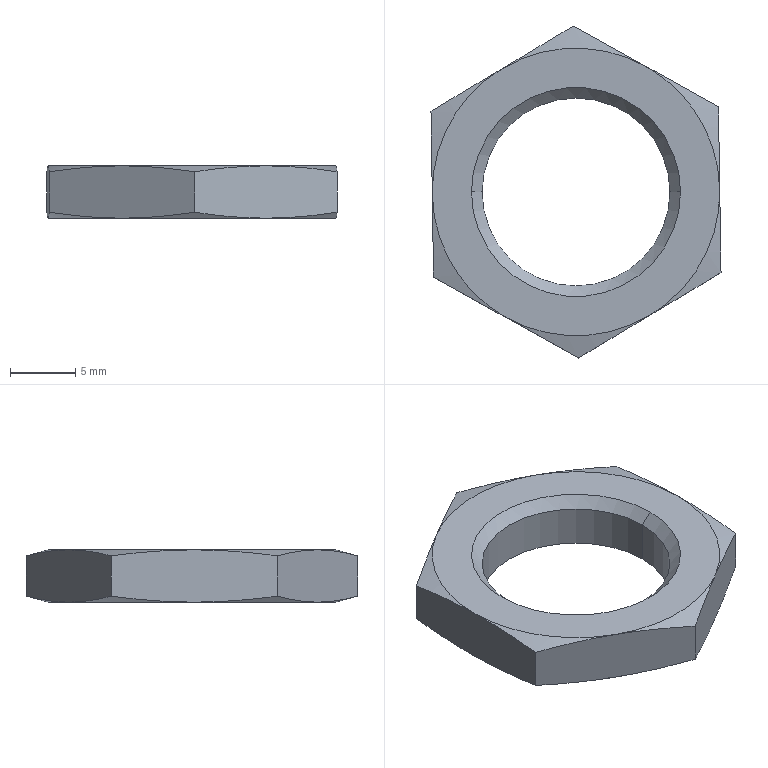Part | SolidWorks | features BaseBody 1 | 1 solid | 25 faces | box 22.195 x 25.4 x 4 mm | volume 1001 mm3 | cone 15 | plane 8 | cylinder 2 | commonest cylinder face diameters 14.376 x2
STEP:
#1=CARTESIAN_POINT('',(71.,0.,357.481));
#2=VERTEX_POINT('',#1);
#3=CARTESIAN_POINT('',(65.648,-9.44,357.481));
#4=VERTEX_POINT('',#3);
#5=CARTESIAN_POINT('',(60.,0.,357.481));
#6=DIRECTION('',(0.,0.,-1.));
#7=DIRECTION('',(1.,0.,0.));
#8=AXIS2_PLACEMENT_3D('',#5,#6,#7);
#9=CIRCLE('',#8,11.);
#10=EDGE_CURVE('',#2,#4,#9,.T.);
#11=ORIENTED_EDGE('',*,*,#10,.F.);
#12=CARTESIAN_POINT('',(71.001,0.,357.481));
#13=VERTEX_POINT('',#12);
#14=CARTESIAN_POINT('',(72.712,0.,357.94));
#15=DIRECTION('',(0.9659,0.,0.2588));
#16=VECTOR('',#15,1000.);
#17=LINE('',#14,#16);
#18=EDGE_CURVE('',#2,#13,#17,.T.);
#19=ORIENTED_EDGE('',*,*,#18,.T.);
#20=CARTESIAN_POINT('',(71.098,-6.179,357.937));
#21=VERTEX_POINT('',#20);
#22=CARTESIAN_POINT('',(71.001,0.,357.481));
#23=CARTESIAN_POINT('',(71.017,-1.035,357.486));
#24=CARTESIAN_POINT('',(71.034,-2.067,357.53));
#25=CARTESIAN_POINT('',(71.066,-4.126,357.687));
#26=CARTESIAN_POINT('',(71.082,-5.153,357.8));
#27=CARTESIAN_POINT('',(71.098,-6.179,357.937));
#28=B_SPLINE_CURVE_WITH_KNOTS('',3,(#22,#23,#24,#25,#26,#27),.UNSPECIFIED.,.F.,.F.,(4,2,4),(0.0001708,0.003269,0.006367),.UNSPECIFIED.);
#29=EDGE_CURVE('',#13,#21,#28,.T.);
#30=ORIENTED_EDGE('',*,*,#29,.T.);
#31=CARTESIAN_POINT('',(71.098,-6.179,357.937));
#32=CARTESIAN_POINT('',(70.193,-6.72,357.796));
#33=CARTESIAN_POINT('',(69.287,-7.262,357.681));
#34=CARTESIAN_POINT('',(67.471,-8.349,357.523));
#35=CARTESIAN_POINT('',(66.561,-8.893,357.481));
#36=CARTESIAN_POINT('',(65.648,-9.44,357.481));
#37=B_SPLINE_CURVE_WITH_KNOTS('',3,(#31,#32,#33,#34,#35,#36),.UNSPECIFIED.,.F.,.F.,(4,2,4),(0.,0.003184,0.006367),.UNSPECIFIED.);
#38=EDGE_CURVE('',#21,#4,#37,.T.);
#39=ORIENTED_EDGE('',*,*,#38,.T.);
#40=EDGE_LOOP('',(#11,#19,#30,#39));
#41=FACE_OUTER_BOUND('',#40,.T.);
#42=CARTESIAN_POINT('',(60.,0.,357.94));
#43=DIRECTION('',(0.,0.,1.));
#44=DIRECTION('',(1.,0.,0.));
#45=AXIS2_PLACEMENT_3D('',#42,#43,#44);
#46=CONICAL_SURFACE('',#45,12.712,1.309);
#47=ADVANCED_FACE('',(#41),#46,.T.);
#48=CARTESIAN_POINT('',(52.812,0.,357.481));
#49=VERTEX_POINT('',#48);
#50=CARTESIAN_POINT('',(67.188,0.,357.481));
#51=VERTEX_POINT('',#50);
#52=CARTESIAN_POINT('',(60.,0.,357.481));
#53=DIRECTION('',(0.,0.,1.));
#54=DIRECTION('',(1.,0.,0.));
#55=AXIS2_PLACEMENT_3D('',#52,#53,#54);
#56=CIRCLE('',#55,7.188);
#57=EDGE_CURVE('',#49,#51,#56,.T.);
#58=ORIENTED_EDGE('',*,*,#57,.F.);
#59=CARTESIAN_POINT('',(52.812,0.,360.669));
#60=VERTEX_POINT('',#59);
#61=CARTESIAN_POINT('',(52.812,0.,358.481));
#62=DIRECTION('',(0.,0.,1.));
#63=VECTOR('',#62,1000.);
#64=LINE('',#61,#63);
#65=EDGE_CURVE('',#49,#60,#64,.T.);
#66=ORIENTED_EDGE('',*,*,#65,.T.);
#67=CARTESIAN_POINT('',(67.188,0.,360.669));
#68=VERTEX_POINT('',#67);
#69=CARTESIAN_POINT('',(60.,0.,360.669));
#70=DIRECTION('',(0.,0.,-1.));
#71=DIRECTION('',(1.,0.,0.));
#72=AXIS2_PLACEMENT_3D('',#69,#70,#71);
#73=CIRCLE('',#72,7.188);
#74=EDGE_CURVE('',#68,#60,#73,.T.);
#75=ORIENTED_EDGE('',*,*,#74,.F.);
#76=CARTESIAN_POINT('',(67.188,0.,358.481));
#77=DIRECTION('',(0.,0.,1.));
#78=VECTOR('',#77,1000.);
#79=LINE('',#76,#78);
#80=EDGE_CURVE('',#51,#68,#79,.T.);
#81=ORIENTED_EDGE('',*,*,#80,.F.);
#82=EDGE_LOOP('',(#58,#66,#75,#81));
#83=FACE_OUTER_BOUND('',#82,.T.);
#84=CARTESIAN_POINT('',(60.,0.,358.481));
#85=DIRECTION('',(0.,0.,1.));
#86=DIRECTION('',(1.,0.,0.));
#87=AXIS2_PLACEMENT_3D('',#84,#85,#86);
#88=CYLINDRICAL_SURFACE('',#87,7.188);
#89=ADVANCED_FACE('',(#83),#88,.F.);
#90=ORIENTED_EDGE('',*,*,#74,.T.);
#91=CARTESIAN_POINT('',(52.,0.,361.481));
#92=VERTEX_POINT('',#91);
#93=CARTESIAN_POINT('',(52.,0.,361.481));
#94=DIRECTION('',(-0.7071,0.,0.7071));
#95=VECTOR('',#94,1000.);
#96=LINE('',#93,#95);
#97=EDGE_CURVE('',#60,#92,#96,.T.);
#98=ORIENTED_EDGE('',*,*,#97,.T.);
#99=CARTESIAN_POINT('',(68.,0.,361.481));
#100=VERTEX_POINT('',#99);
#101=CARTESIAN_POINT('',(60.,0.,361.481));
#102=DIRECTION('',(0.,0.,-1.));
#103=DIRECTION('',(1.,0.,0.));
#104=AXIS2_PLACEMENT_3D('',#101,#102,#103);
#105=CIRCLE('',#104,8.);
#106=EDGE_CURVE('',#100,#92,#105,.T.);
#107=ORIENTED_EDGE('',*,*,#106,.F.);
#108=CARTESIAN_POINT('',(68.,0.,361.481));
#109=DIRECTION('',(0.7071,0.,0.7071));
#110=VECTOR('',#109,1000.);
#111=LINE('',#108,#110);
#112=EDGE_CURVE('',#68,#100,#111,.T.);
#113=ORIENTED_EDGE('',*,*,#112,.F.);
#114=EDGE_LOOP('',(#90,#98,#107,#113));
#115=FACE_OUTER_BOUND('',#114,.T.);
#116=CARTESIAN_POINT('',(60.,0.,361.481));
#117=DIRECTION('',(0.,0.,1.));
#118=DIRECTION('',(1.,0.,0.));
#119=AXIS2_PLACEMENT_3D('',#116,#117,#118);
#120=CONICAL_SURFACE('',#119,8.,0.7854);
#121=ADVANCED_FACE('',(#115),#120,.F.);
#122=CARTESIAN_POINT('',(70.999,0.1712,357.481));
#123=VERTEX_POINT('',#122);
#124=CARTESIAN_POINT('',(60.,0.,357.481));
#125=DIRECTION('',(0.,0.,-1.));
#126=DIRECTION('',(1.,0.,0.));
#127=AXIS2_PLACEMENT_3D('',#124,#125,#126);
#128=CIRCLE('',#127,11.);
#129=EDGE_CURVE('',#123,#2,#128,.T.);
#130=ORIENTED_EDGE('',*,*,#129,.T.);
#131=ORIENTED_EDGE('',*,*,#10,.T.);
#132=CARTESIAN_POINT('',(54.649,-9.611,357.481));
#133=VERTEX_POINT('',#132);
#134=CARTESIAN_POINT('',(60.,0.,357.481));
#135=DIRECTION('',(0.,0.,-1.));
#136=DIRECTION('',(1.,0.,0.));
#137=AXIS2_PLACEMENT_3D('',#134,#135,#136);
#138=CIRCLE('',#137,11.);
#139=EDGE_CURVE('',#4,#133,#138,.T.);
#140=ORIENTED_EDGE('',*,*,#139,.T.);
#141=CARTESIAN_POINT('',(49.001,-0.1712,357.481));
#142=VERTEX_POINT('',#141);
#143=CARTESIAN_POINT('',(60.,0.,357.481));
#144=DIRECTION('',(0.,0.,-1.));
#145=DIRECTION('',(1.,0.,0.));
#146=AXIS2_PLACEMENT_3D('',#143,#144,#145);
#147=CIRCLE('',#146,11.);
#148=EDGE_CURVE('',#133,#142,#147,.T.);
#149=ORIENTED_EDGE('',*,*,#148,.T.);
#150=CARTESIAN_POINT('',(54.352,9.44,357.481));
#151=VERTEX_POINT('',#150);
#152=CARTESIAN_POINT('',(60.,0.,357.481));
#153=DIRECTION('',(0.,0.,-1.));
#154=DIRECTION('',(1.,0.,0.));
#155=AXIS2_PLACEMENT_3D('',#152,#153,#154);
#156=CIRCLE('',#155,11.);
#157=EDGE_CURVE('',#142,#151,#156,.T.);
#158=ORIENTED_EDGE('',*,*,#157,.T.);
#159=CARTESIAN_POINT('',(65.351,9.611,357.481));
#160=VERTEX_POINT('',#159);
#161=CARTESIAN_POINT('',(60.,0.,357.481));
#162=DIRECTION('',(0.,0.,-1.));
#163=DIRECTION('',(1.,0.,0.));
#164=AXIS2_PLACEMENT_3D('',#161,#162,#163);
#165=CIRCLE('',#164,11.);
#166=EDGE_CURVE('',#151,#160,#165,.T.);
#167=ORIENTED_EDGE('',*,*,#166,.T.);
#168=CARTESIAN_POINT('',(60.,0.,357.481));
#169=DIRECTION('',(0.,0.,-1.));
#170=DIRECTION('',(1.,0.,0.));
#171=AXIS2_PLACEMENT_3D('',#168,#169,#170);
#172=CIRCLE('',#171,11.);
#173=EDGE_CURVE('',#160,#123,#172,.T.);
#174=ORIENTED_EDGE('',*,*,#173,.T.);
#175=EDGE_LOOP('',(#130,#131,#140,#149,#158,#167,#174));
#176=FACE_OUTER_BOUND('',#175,.T.);
#177=CARTESIAN_POINT('',(60.,0.,357.481));
#178=DIRECTION('',(0.,0.,1.));
#179=DIRECTION('',(1.,0.,0.));
#180=AXIS2_PLACEMENT_3D('',#177,#178,#179);
#181=CIRCLE('',#180,7.188);
#182=EDGE_CURVE('',#51,#49,#181,.T.);
#183=ORIENTED_EDGE('',*,*,#182,.T.);
#184=ORIENTED_EDGE('',*,*,#57,.T.);
#185=EDGE_LOOP('',(#183,#184));
#186=FACE_BOUND('',#185,.T.);
#187=CARTESIAN_POINT('',(55.123,8.152,357.481));
#188=DIRECTION('',(0.,0.,-1.));
#189=DIRECTION('',(-1.,0.,0.));
#190=AXIS2_PLACEMENT_3D('',#187,#188,#189);
#191=PLANE('',#190);
#192=ADVANCED_FACE('',(#176,#186),#191,.T.);
#193=CARTESIAN_POINT('',(60.198,-12.7,357.937));
#194=VERTEX_POINT('',#193);
#195=CARTESIAN_POINT('',(65.648,-9.44,357.481));
#196=CARTESIAN_POINT('',(64.735,-9.986,357.481));
#197=CARTESIAN_POINT('',(63.824,-10.53,357.523));
#198=CARTESIAN_POINT('',(62.008,-11.617,357.681));
#199=CARTESIAN_POINT('',(61.102,-12.159,357.796));
#200=CARTESIAN_POINT('',(60.198,-12.7,357.937));
#201=B_SPLINE_CURVE_WITH_KNOTS('',3,(#195,#196,#197,#198,#199,#200),.UNSPECIFIED.,.F.,.F.,(4,2,4),(0.,0.003184,0.006367),.UNSPECIFIED.);
#202=EDGE_CURVE('',#4,#194,#201,.T.);
#203=ORIENTED_EDGE('',*,*,#202,.T.);
#204=CARTESIAN_POINT('',(60.198,-12.7,357.937));
#205=CARTESIAN_POINT('',(59.277,-12.188,357.796));
#206=CARTESIAN_POINT('',(58.355,-11.674,357.681));
#207=CARTESIAN_POINT('',(56.505,-10.644,357.523));
#208=CARTESIAN_POINT('',(55.579,-10.128,357.481));
#209=CARTESIAN_POINT('',(54.649,-9.611,357.481));
#210=B_SPLINE_CURVE_WITH_KNOTS('',3,(#204,#205,#206,#207,#208,#209),.UNSPECIFIED.,.F.,.F.,(4,2,4),(0.,0.003184,0.006367),.UNSPECIFIED.);
#211=EDGE_CURVE('',#194,#133,#210,.T.);
#212=ORIENTED_EDGE('',*,*,#211,.T.);
#213=ORIENTED_EDGE('',*,*,#139,.F.);
#214=EDGE_LOOP('',(#203,#212,#213));
#215=FACE_OUTER_BOUND('',#214,.T.);
#216=CARTESIAN_POINT('',(60.,0.,357.94));
#217=DIRECTION('',(0.,0.,1.));
#218=DIRECTION('',(1.,0.,0.));
#219=AXIS2_PLACEMENT_3D('',#216,#217,#218);
#220=CONICAL_SURFACE('',#219,12.712,1.309);
#221=ADVANCED_FACE('',(#215),#220,.T.);
#222=ORIENTED_EDGE('',*,*,#18,.F.);
#223=ORIENTED_EDGE('',*,*,#129,.F.);
#224=CARTESIAN_POINT('',(70.999,0.1712,357.481));
#225=CARTESIAN_POINT('',(71.,0.1141,357.481));
#226=CARTESIAN_POINT('',(71.,0.05707,357.481));
#227=CARTESIAN_POINT('',(71.001,0.,357.481));
#228=B_SPLINE_CURVE_WITH_KNOTS('',3,(#224,#225,#226,#227),.UNSPECIFIED.,.F.,.F.,(4,4),(0.,0.0001708),.UNSPECIFIED.);
#229=EDGE_CURVE('',#123,#13,#228,.T.);
#230=ORIENTED_EDGE('',*,*,#229,.T.);
#231=EDGE_LOOP('',(#222,#223,#230));
#232=FACE_OUTER_BOUND('',#231,.T.);
#233=CARTESIAN_POINT('',(60.,0.,357.94));
#234=DIRECTION('',(0.,0.,1.));
#235=DIRECTION('',(1.,0.,0.));
#236=AXIS2_PLACEMENT_3D('',#233,#234,#235);
#237=CONICAL_SURFACE('',#236,12.712,1.309);
#238=ADVANCED_FACE('',(#232),#237,.T.);
#239=CARTESIAN_POINT('',(70.9,6.521,357.937));
#240=VERTEX_POINT('',#239);
#241=CARTESIAN_POINT('',(70.9,6.521,357.937));
#242=CARTESIAN_POINT('',(70.916,5.468,357.796));
#243=CARTESIAN_POINT('',(70.933,4.412,357.681));
#244=CARTESIAN_POINT('',(70.966,2.296,357.523));
#245=CARTESIAN_POINT('',(70.982,1.235,357.481));
#246=CARTESIAN_POINT('',(70.999,0.1712,357.481));
#247=B_SPLINE_CURVE_WITH_KNOTS('',3,(#241,#242,#243,#244,#245,#246),.UNSPECIFIED.,.F.,.F.,(4,2,4),(0.,0.003184,0.006367),.UNSPECIFIED.);
#248=EDGE_CURVE('',#240,#123,#247,.T.);
#249=ORIENTED_EDGE('',*,*,#248,.T.);
#250=ORIENTED_EDGE('',*,*,#173,.F.);
#251=CARTESIAN_POINT('',(65.351,9.611,357.481));
#252=CARTESIAN_POINT('',(66.281,9.093,357.481));
#253=CARTESIAN_POINT('',(67.208,8.577,357.523));
#254=CARTESIAN_POINT('',(69.057,7.547,357.681));
#255=CARTESIAN_POINT('',(69.979,7.034,357.796));
#256=CARTESIAN_POINT('',(70.9,6.521,357.937));
#257=B_SPLINE_CURVE_WITH_KNOTS('',3,(#251,#252,#253,#254,#255,#256),.UNSPECIFIED.,.F.,.F.,(4,2,4),(0.,0.003184,0.006367),.UNSPECIFIED.);
#258=EDGE_CURVE('',#160,#240,#257,.T.);
#259=ORIENTED_EDGE('',*,*,#258,.T.);
#260=EDGE_LOOP('',(#249,#250,#259));
#261=FACE_OUTER_BOUND('',#260,.T.);
#262=CARTESIAN_POINT('',(60.,0.,357.94));
#263=DIRECTION('',(0.,0.,1.));
#264=DIRECTION('',(1.,0.,0.));
#265=AXIS2_PLACEMENT_3D('',#262,#263,#264);
#266=CONICAL_SURFACE('',#265,12.712,1.309);
#267=ADVANCED_FACE('',(#261),#266,.T.);
#268=ORIENTED_EDGE('',*,*,#166,.F.);
#269=CARTESIAN_POINT('',(59.802,12.7,357.937));
#270=VERTEX_POINT('',#269);
#271=CARTESIAN_POINT('',(54.352,9.44,357.481));
#272=CARTESIAN_POINT('',(55.265,9.986,357.481));
#273=CARTESIAN_POINT('',(56.176,10.53,357.523));
#274=CARTESIAN_POINT('',(57.992,11.617,357.681));
#275=CARTESIAN_POINT('',(58.898,12.159,357.796));
#276=CARTESIAN_POINT('',(59.802,12.7,357.937));
#277=B_SPLINE_CURVE_WITH_KNOTS('',3,(#271,#272,#273,#274,#275,#276),.UNSPECIFIED.,.F.,.F.,(4,2,4),(0.,0.003184,0.006367),.UNSPECIFIED.);
#278=EDGE_CURVE('',#151,#270,#277,.T.);
#279=ORIENTED_EDGE('',*,*,#278,.T.);
#280=CARTESIAN_POINT('',(59.802,12.7,357.937));
#281=CARTESIAN_POINT('',(60.723,12.188,357.796));
#282=CARTESIAN_POINT('',(61.645,11.674,357.681));
#283=CARTESIAN_POINT('',(63.495,10.644,357.523));
#284=CARTESIAN_POINT('',(64.421,10.128,357.481));
#285=CARTESIAN_POINT('',(65.351,9.611,357.481));
#286=B_SPLINE_CURVE_WITH_KNOTS('',3,(#280,#281,#282,#283,#284,#285),.UNSPECIFIED.,.F.,.F.,(4,2,4),(0.,0.003184,0.006367),.UNSPECIFIED.);
#287=EDGE_CURVE('',#270,#160,#286,.T.);
#288=ORIENTED_EDGE('',*,*,#287,.T.);
#289=EDGE_LOOP('',(#268,#279,#288));
#290=FACE_OUTER_BOUND('',#289,.T.);
#291=CARTESIAN_POINT('',(60.,0.,357.94));
#292=DIRECTION('',(0.,0.,1.));
#293=DIRECTION('',(1.,0.,0.));
#294=AXIS2_PLACEMENT_3D('',#291,#292,#293);
#295=CONICAL_SURFACE('',#294,12.712,1.309);
#296=ADVANCED_FACE('',(#290),#295,.T.);
#297=CARTESIAN_POINT('',(48.902,6.179,357.937));
#298=VERTEX_POINT('',#297);
#299=CARTESIAN_POINT('',(49.001,-0.1712,357.481));
#300=CARTESIAN_POINT('',(48.985,0.8926,357.481));
#301=CARTESIAN_POINT('',(48.968,1.953,357.523));
#302=CARTESIAN_POINT('',(48.935,4.07,357.681));
#303=CARTESIAN_POINT('',(48.919,5.125,357.796));
#304=CARTESIAN_POINT('',(48.902,6.179,357.937));
#305=B_SPLINE_CURVE_WITH_KNOTS('',3,(#299,#300,#301,#302,#303,#304),.UNSPECIFIED.,.F.,.F.,(4,2,4),(0.,0.003184,0.006367),.UNSPECIFIED.);
#306=EDGE_CURVE('',#142,#298,#305,.T.);
#307=ORIENTED_EDGE('',*,*,#306,.T.);
#308=CARTESIAN_POINT('',(48.902,6.179,357.937));
#309=CARTESIAN_POINT('',(49.807,6.72,357.796));
#310=CARTESIAN_POINT('',(50.713,7.262,357.681));
#311=CARTESIAN_POINT('',(52.529,8.349,357.523));
#312=CARTESIAN_POINT('',(53.439,8.893,357.481));
#313=CARTESIAN_POINT('',(54.352,9.44,357.481));
#314=B_SPLINE_CURVE_WITH_KNOTS('',3,(#308,#309,#310,#311,#312,#313),.UNSPECIFIED.,.F.,.F.,(4,2,4),(0.,0.003184,0.006367),.UNSPECIFIED.);
#315=EDGE_CURVE('',#298,#151,#314,.T.);
#316=ORIENTED_EDGE('',*,*,#315,.T.);
#317=ORIENTED_EDGE('',*,*,#157,.F.);
#318=EDGE_LOOP('',(#307,#316,#317));
#319=FACE_OUTER_BOUND('',#318,.T.);
#320=CARTESIAN_POINT('',(60.,0.,357.94));
#321=DIRECTION('',(0.,0.,1.));
#322=DIRECTION('',(1.,0.,0.));
#323=AXIS2_PLACEMENT_3D('',#320,#321,#322);
#324=CONICAL_SURFACE('',#323,12.712,1.309);
#325=ADVANCED_FACE('',(#319),#324,.T.);
#326=CARTESIAN_POINT('',(49.1,-6.521,357.937));
#327=VERTEX_POINT('',#326);
#328=CARTESIAN_POINT('',(54.649,-9.611,357.481));
#329=CARTESIAN_POINT('',(53.719,-9.093,357.481));
#330=CARTESIAN_POINT('',(52.792,-8.577,357.523));
#331=CARTESIAN_POINT('',(50.943,-7.547,357.681));
#332=CARTESIAN_POINT('',(50.021,-7.034,357.796));
#333=CARTESIAN_POINT('',(49.1,-6.521,357.937));
#334=B_SPLINE_CURVE_WITH_KNOTS('',3,(#328,#329,#330,#331,#332,#333),.UNSPECIFIED.,.F.,.F.,(4,2,4),(0.,0.003184,0.006367),.UNSPECIFIED.);
#335=EDGE_CURVE('',#133,#327,#334,.T.);
#336=ORIENTED_EDGE('',*,*,#335,.T.);
#337=CARTESIAN_POINT('',(49.1,-6.521,357.937));
#338=CARTESIAN_POINT('',(49.084,-5.468,357.796));
#339=CARTESIAN_POINT('',(49.067,-4.412,357.681));
#340=CARTESIAN_POINT('',(49.034,-2.296,357.523));
#341=CARTESIAN_POINT('',(49.018,-1.235,357.481));
#342=CARTESIAN_POINT('',(49.001,-0.1712,357.481));
#343=B_SPLINE_CURVE_WITH_KNOTS('',3,(#337,#338,#339,#340,#341,#342),.UNSPECIFIED.,.F.,.F.,(4,2,4),(0.,0.003184,0.006367),.UNSPECIFIED.);
#344=EDGE_CURVE('',#327,#142,#343,.T.);
#345=ORIENTED_EDGE('',*,*,#344,.T.);
#346=ORIENTED_EDGE('',*,*,#148,.F.);
#347=EDGE_LOOP('',(#336,#345,#346));
#348=FACE_OUTER_BOUND('',#347,.T.);
#349=CARTESIAN_POINT('',(60.,0.,357.94));
#350=DIRECTION('',(0.,0.,1.));
#351=DIRECTION('',(1.,0.,0.));
#352=AXIS2_PLACEMENT_3D('',#349,#350,#351);
#353=CONICAL_SURFACE('',#352,12.712,1.309);
#354=ADVANCED_FACE('',(#348),#353,.T.);
#355=ORIENTED_EDGE('',*,*,#65,.F.);
#356=ORIENTED_EDGE('',*,*,#182,.F.);
#357=ORIENTED_EDGE('',*,*,#80,.T.);
#358=CARTESIAN_POINT('',(60.,0.,360.669));
#359=DIRECTION('',(0.,0.,-1.));
#360=DIRECTION('',(1.,0.,0.));
#361=AXIS2_PLACEMENT_3D('',#358,#359,#360);
#362=CIRCLE('',#361,7.188);
#363=EDGE_CURVE('',#60,#68,#362,.T.);
#364=ORIENTED_EDGE('',*,*,#363,.F.);
#365=EDGE_LOOP('',(#355,#356,#357,#364));
#366=FACE_OUTER_BOUND('',#365,.T.);
#367=CARTESIAN_POINT('',(60.,0.,358.481));
#368=DIRECTION('',(0.,0.,1.));
#369=DIRECTION('',(1.,0.,0.));
#370=AXIS2_PLACEMENT_3D('',#367,#368,#369);
#371=CYLINDRICAL_SURFACE('',#370,7.188);
#372=ADVANCED_FACE('',(#366),#371,.F.);
#373=ORIENTED_EDGE('',*,*,#335,.F.);
#374=ORIENTED_EDGE('',*,*,#211,.F.);
#375=CARTESIAN_POINT('',(60.198,-12.7,361.025));
#376=VERTEX_POINT('',#375);
#377=CARTESIAN_POINT('',(60.198,-12.7,355.481));
#378=DIRECTION('',(0.,0.,-1.));
#379=VECTOR('',#378,1000.);
#380=LINE('',#377,#379);
#381=EDGE_CURVE('',#376,#194,#380,.T.);
#382=ORIENTED_EDGE('',*,*,#381,.F.);
#383=CARTESIAN_POINT('',(54.649,-9.611,361.481));
#384=VERTEX_POINT('',#383);
#385=CARTESIAN_POINT('',(54.649,-9.611,361.481));
#386=CARTESIAN_POINT('',(55.579,-10.128,361.481));
#387=CARTESIAN_POINT('',(56.505,-10.644,361.439));
#388=CARTESIAN_POINT('',(58.355,-11.674,361.281));
#389=CARTESIAN_POINT('',(59.277,-12.188,361.166));
#390=CARTESIAN_POINT('',(60.198,-12.7,361.025));
#391=B_SPLINE_CURVE_WITH_KNOTS('',3,(#385,#386,#387,#388,#389,#390),.UNSPECIFIED.,.F.,.F.,(4,2,4),(0.,0.003184,0.006367),.UNSPECIFIED.);
#392=EDGE_CURVE('',#384,#376,#391,.T.);
#393=ORIENTED_EDGE('',*,*,#392,.F.);
#394=CARTESIAN_POINT('',(49.1,-6.521,361.025));
#395=VERTEX_POINT('',#394);
#396=CARTESIAN_POINT('',(49.1,-6.521,361.025));
#397=CARTESIAN_POINT('',(50.021,-7.034,361.166));
#398=CARTESIAN_POINT('',(50.943,-7.547,361.281));
#399=CARTESIAN_POINT('',(52.792,-8.577,361.439));
#400=CARTESIAN_POINT('',(53.719,-9.093,361.481));
#401=CARTESIAN_POINT('',(54.649,-9.611,361.481));
#402=B_SPLINE_CURVE_WITH_KNOTS('',3,(#396,#397,#398,#399,#400,#401),.UNSPECIFIED.,.F.,.F.,(4,2,4),(0.,0.003184,0.006367),.UNSPECIFIED.);
#403=EDGE_CURVE('',#395,#384,#402,.T.);
#404=ORIENTED_EDGE('',*,*,#403,.F.);
#405=CARTESIAN_POINT('',(49.1,-6.521,355.481));
#406=DIRECTION('',(0.,0.,1.));
#407=VECTOR('',#406,1000.);
#408=LINE('',#405,#407);
#409=EDGE_CURVE('',#327,#395,#408,.T.);
#410=ORIENTED_EDGE('',*,*,#409,.F.);
#411=EDGE_LOOP('',(#373,#374,#382,#393,#404,#410));
#412=FACE_OUTER_BOUND('',#411,.T.);
#413=CARTESIAN_POINT('',(49.1,-6.521,355.481));
#414=DIRECTION('',(0.4865,0.8737,0.));
#415=DIRECTION('',(-0.8737,0.4865,0.));
#416=AXIS2_PLACEMENT_3D('',#413,#414,#415);
#417=PLANE('',#416);
#418=ADVANCED_FACE('',(#412),#417,.F.);
#419=ORIENTED_EDGE('',*,*,#202,.F.);
#420=ORIENTED_EDGE('',*,*,#38,.F.);
#421=CARTESIAN_POINT('',(71.098,-6.179,361.025));
#422=VERTEX_POINT('',#421);
#423=CARTESIAN_POINT('',(71.098,-6.179,355.481));
#424=DIRECTION('',(0.,0.,-1.));
#425=VECTOR('',#424,1000.);
#426=LINE('',#423,#425);
#427=EDGE_CURVE('',#422,#21,#426,.T.);
#428=ORIENTED_EDGE('',*,*,#427,.F.);
#429=CARTESIAN_POINT('',(65.648,-9.44,361.481));
#430=VERTEX_POINT('',#429);
#431=CARTESIAN_POINT('',(65.648,-9.44,361.481));
#432=CARTESIAN_POINT('',(66.561,-8.893,361.481));
#433=CARTESIAN_POINT('',(67.471,-8.349,361.439));
#434=CARTESIAN_POINT('',(69.287,-7.262,361.281));
#435=CARTESIAN_POINT('',(70.193,-6.72,361.166));
#436=CARTESIAN_POINT('',(71.098,-6.179,361.025));
#437=B_SPLINE_CURVE_WITH_KNOTS('',3,(#431,#432,#433,#434,#435,#436),.UNSPECIFIED.,.F.,.F.,(4,2,4),(0.,0.003184,0.006367),.UNSPECIFIED.);
#438=EDGE_CURVE('',#430,#422,#437,.T.);
#439=ORIENTED_EDGE('',*,*,#438,.F.);
#440=CARTESIAN_POINT('',(60.198,-12.7,361.025));
#441=CARTESIAN_POINT('',(61.102,-12.159,361.166));
#442=CARTESIAN_POINT('',(62.008,-11.617,361.281));
#443=CARTESIAN_POINT('',(63.824,-10.53,361.439));
#444=CARTESIAN_POINT('',(64.735,-9.986,361.481));
#445=CARTESIAN_POINT('',(65.648,-9.44,361.481));
#446=B_SPLINE_CURVE_WITH_KNOTS('',3,(#440,#441,#442,#443,#444,#445),.UNSPECIFIED.,.F.,.F.,(4,2,4),(0.,0.003184,0.006367),.UNSPECIFIED.);
#447=EDGE_CURVE('',#376,#430,#446,.T.);
#448=ORIENTED_EDGE('',*,*,#447,.F.);
#449=ORIENTED_EDGE('',*,*,#381,.T.);
#450=EDGE_LOOP('',(#419,#420,#428,#439,#448,#449));
#451=FACE_OUTER_BOUND('',#450,.T.);
#452=CARTESIAN_POINT('',(60.198,-12.7,355.481));
#453=DIRECTION('',(-0.5134,0.8581,0.));
#454=DIRECTION('',(-0.8581,-0.5134,0.));
#455=AXIS2_PLACEMENT_3D('',#452,#453,#454);
#456=PLANE('',#455);
#457=ADVANCED_FACE('',(#451),#456,.F.);
#458=ORIENTED_EDGE('',*,*,#229,.F.);
#459=ORIENTED_EDGE('',*,*,#248,.F.);
#460=CARTESIAN_POINT('',(70.9,6.521,361.025));
#461=VERTEX_POINT('',#460);
#462=CARTESIAN_POINT('',(70.9,6.521,355.481));
#463=DIRECTION('',(0.,0.,-1.));
#464=VECTOR('',#463,1000.);
#465=LINE('',#462,#464);
#466=EDGE_CURVE('',#461,#240,#465,.T.);
#467=ORIENTED_EDGE('',*,*,#466,.F.);
#468=CARTESIAN_POINT('',(70.999,0.1712,361.481));
#469=VERTEX_POINT('',#468);
#470=CARTESIAN_POINT('',(70.999,0.1712,361.481));
#471=CARTESIAN_POINT('',(70.982,1.235,361.481));
#472=CARTESIAN_POINT('',(70.966,2.296,361.439));
#473=CARTESIAN_POINT('',(70.933,4.412,361.281));
#474=CARTESIAN_POINT('',(70.916,5.468,361.166));
#475=CARTESIAN_POINT('',(70.9,6.521,361.025));
#476=B_SPLINE_CURVE_WITH_KNOTS('',3,(#470,#471,#472,#473,#474,#475),.UNSPECIFIED.,.F.,.F.,(4,2,4),(0.,0.003184,0.006367),.UNSPECIFIED.);
#477=EDGE_CURVE('',#469,#461,#476,.T.);
#478=ORIENTED_EDGE('',*,*,#477,.F.);
#479=CARTESIAN_POINT('',(71.098,-6.179,361.025));
#480=CARTESIAN_POINT('',(71.081,-5.125,361.166));
#481=CARTESIAN_POINT('',(71.065,-4.07,361.281));
#482=CARTESIAN_POINT('',(71.032,-1.953,361.439));
#483=CARTESIAN_POINT('',(71.015,-0.8926,361.481));
#484=CARTESIAN_POINT('',(70.999,0.1712,361.481));
#485=B_SPLINE_CURVE_WITH_KNOTS('',3,(#479,#480,#481,#482,#483,#484),.UNSPECIFIED.,.F.,.F.,(4,2,4),(0.,0.003184,0.006367),.UNSPECIFIED.);
#486=EDGE_CURVE('',#422,#469,#485,.T.);
#487=ORIENTED_EDGE('',*,*,#486,.F.);
#488=ORIENTED_EDGE('',*,*,#427,.T.);
#489=ORIENTED_EDGE('',*,*,#29,.F.);
#490=EDGE_LOOP('',(#458,#459,#467,#478,#487,#488,#489));
#491=FACE_OUTER_BOUND('',#490,.T.);
#492=CARTESIAN_POINT('',(71.098,-6.179,355.481));
#493=DIRECTION('',(-0.9999,-0.01557,0.));
#494=DIRECTION('',(0.01557,-0.9999,0.));
#495=AXIS2_PLACEMENT_3D('',#492,#493,#494);
#496=PLANE('',#495);
#497=ADVANCED_FACE('',(#491),#496,.F.);
#498=ORIENTED_EDGE('',*,*,#466,.T.);
#499=ORIENTED_EDGE('',*,*,#258,.F.);
#500=ORIENTED_EDGE('',*,*,#287,.F.);
#501=CARTESIAN_POINT('',(59.802,12.7,361.025));
#502=VERTEX_POINT('',#501);
#503=CARTESIAN_POINT('',(59.802,12.7,355.481));
#504=DIRECTION('',(0.,0.,-1.));
#505=VECTOR('',#504,1000.);
#506=LINE('',#503,#505);
#507=EDGE_CURVE('',#502,#270,#506,.T.);
#508=ORIENTED_EDGE('',*,*,#507,.F.);
#509=CARTESIAN_POINT('',(65.351,9.611,361.481));
#510=VERTEX_POINT('',#509);
#511=CARTESIAN_POINT('',(65.351,9.611,361.481));
#512=CARTESIAN_POINT('',(64.421,10.128,361.481));
#513=CARTESIAN_POINT('',(63.495,10.644,361.439));
#514=CARTESIAN_POINT('',(61.645,11.674,361.281));
#515=CARTESIAN_POINT('',(60.723,12.188,361.166));
#516=CARTESIAN_POINT('',(59.802,12.7,361.025));
#517=B_SPLINE_CURVE_WITH_KNOTS('',3,(#511,#512,#513,#514,#515,#516),.UNSPECIFIED.,.F.,.F.,(4,2,4),(0.,0.003184,0.006367),.UNSPECIFIED.);
#518=EDGE_CURVE('',#510,#502,#517,.T.);
#519=ORIENTED_EDGE('',*,*,#518,.F.);
#520=CARTESIAN_POINT('',(70.9,6.521,361.025));
#521=CARTESIAN_POINT('',(69.979,7.034,361.166));
#522=CARTESIAN_POINT('',(69.057,7.547,361.281));
#523=CARTESIAN_POINT('',(67.208,8.577,361.439));
#524=CARTESIAN_POINT('',(66.281,9.093,361.481));
#525=CARTESIAN_POINT('',(65.351,9.611,361.481));
#526=B_SPLINE_CURVE_WITH_KNOTS('',3,(#520,#521,#522,#523,#524,#525),.UNSPECIFIED.,.F.,.F.,(4,2,4),(0.,0.003184,0.006367),.UNSPECIFIED.);
#527=EDGE_CURVE('',#461,#510,#526,.T.);
#528=ORIENTED_EDGE('',*,*,#527,.F.);
#529=EDGE_LOOP('',(#498,#499,#500,#508,#519,#528));
#530=FACE_OUTER_BOUND('',#529,.T.);
#531=CARTESIAN_POINT('',(70.9,6.521,355.481));
#532=DIRECTION('',(-0.4865,-0.8737,0.));
#533=DIRECTION('',(0.8737,-0.4865,0.));
#534=AXIS2_PLACEMENT_3D('',#531,#532,#533);
#535=PLANE('',#534);
#536=ADVANCED_FACE('',(#530),#535,.F.);
#537=ORIENTED_EDGE('',*,*,#507,.T.);
#538=ORIENTED_EDGE('',*,*,#278,.F.);
#539=ORIENTED_EDGE('',*,*,#315,.F.);
#540=CARTESIAN_POINT('',(48.902,6.179,361.025));
#541=VERTEX_POINT('',#540);
#542=CARTESIAN_POINT('',(48.902,6.179,355.481));
#543=DIRECTION('',(0.,0.,-1.));
#544=VECTOR('',#543,1000.);
#545=LINE('',#542,#544);
#546=EDGE_CURVE('',#541,#298,#545,.T.);
#547=ORIENTED_EDGE('',*,*,#546,.F.);
#548=CARTESIAN_POINT('',(54.352,9.44,361.481));
#549=VERTEX_POINT('',#548);
#550=CARTESIAN_POINT('',(54.352,9.44,361.481));
#551=CARTESIAN_POINT('',(53.439,8.893,361.481));
#552=CARTESIAN_POINT('',(52.529,8.349,361.439));
#553=CARTESIAN_POINT('',(50.713,7.262,361.281));
#554=CARTESIAN_POINT('',(49.807,6.72,361.166));
#555=CARTESIAN_POINT('',(48.902,6.179,361.025));
#556=B_SPLINE_CURVE_WITH_KNOTS('',3,(#550,#551,#552,#553,#554,#555),.UNSPECIFIED.,.F.,.F.,(4,2,4),(0.,0.003184,0.006367),.UNSPECIFIED.);
#557=EDGE_CURVE('',#549,#541,#556,.T.);
#558=ORIENTED_EDGE('',*,*,#557,.F.);
#559=CARTESIAN_POINT('',(59.802,12.7,361.025));
#560=CARTESIAN_POINT('',(58.898,12.159,361.166));
#561=CARTESIAN_POINT('',(57.992,11.617,361.281));
#562=CARTESIAN_POINT('',(56.176,10.53,361.439));
#563=CARTESIAN_POINT('',(55.265,9.986,361.481));
#564=CARTESIAN_POINT('',(54.352,9.44,361.481));
#565=B_SPLINE_CURVE_WITH_KNOTS('',3,(#559,#560,#561,#562,#563,#564),.UNSPECIFIED.,.F.,.F.,(4,2,4),(0.,0.003184,0.006367),.UNSPECIFIED.);
#566=EDGE_CURVE('',#502,#549,#565,.T.);
#567=ORIENTED_EDGE('',*,*,#566,.F.);
#568=EDGE_LOOP('',(#537,#538,#539,#547,#558,#567));
#569=FACE_OUTER_BOUND('',#568,.T.);
#570=CARTESIAN_POINT('',(59.802,12.7,355.481));
#571=DIRECTION('',(0.5134,-0.8581,0.));
#572=DIRECTION('',(0.8581,0.5134,0.));
#573=AXIS2_PLACEMENT_3D('',#570,#571,#572);
#574=PLANE('',#573);
#575=ADVANCED_FACE('',(#569),#574,.F.);
#576=ORIENTED_EDGE('',*,*,#546,.T.);
#577=ORIENTED_EDGE('',*,*,#306,.F.);
#578=ORIENTED_EDGE('',*,*,#344,.F.);
#579=ORIENTED_EDGE('',*,*,#409,.T.);
#580=CARTESIAN_POINT('',(49.001,-0.1712,361.481));
#581=VERTEX_POINT('',#580);
#582=CARTESIAN_POINT('',(49.001,-0.1712,361.481));
#583=CARTESIAN_POINT('',(49.018,-1.235,361.481));
#584=CARTESIAN_POINT('',(49.034,-2.296,361.439));
#585=CARTESIAN_POINT('',(49.067,-4.412,361.281));
#586=CARTESIAN_POINT('',(49.084,-5.468,361.166));
#587=CARTESIAN_POINT('',(49.1,-6.521,361.025));
#588=B_SPLINE_CURVE_WITH_KNOTS('',3,(#582,#583,#584,#585,#586,#587),.UNSPECIFIED.,.F.,.F.,(4,2,4),(0.,0.003184,0.006367),.UNSPECIFIED.);
#589=EDGE_CURVE('',#581,#395,#588,.T.);
#590=ORIENTED_EDGE('',*,*,#589,.F.);
#591=CARTESIAN_POINT('',(48.902,6.179,361.025));
#592=CARTESIAN_POINT('',(48.919,5.125,361.166));
#593=CARTESIAN_POINT('',(48.935,4.07,361.281));
#594=CARTESIAN_POINT('',(48.968,1.953,361.439));
#595=CARTESIAN_POINT('',(48.985,0.8926,361.481));
#596=CARTESIAN_POINT('',(49.001,-0.1712,361.481));
#597=B_SPLINE_CURVE_WITH_KNOTS('',3,(#591,#592,#593,#594,#595,#596),.UNSPECIFIED.,.F.,.F.,(4,2,4),(0.,0.003184,0.006367),.UNSPECIFIED.);
#598=EDGE_CURVE('',#541,#581,#597,.T.);
#599=ORIENTED_EDGE('',*,*,#598,.F.);
#600=EDGE_LOOP('',(#576,#577,#578,#579,#590,#599));
#601=FACE_OUTER_BOUND('',#600,.T.);
#602=CARTESIAN_POINT('',(48.902,6.179,355.481));
#603=DIRECTION('',(0.9999,0.01557,0.));
#604=DIRECTION('',(-0.01557,0.9999,0.));
#605=AXIS2_PLACEMENT_3D('',#602,#603,#604);
#606=PLANE('',#605);
#607=ADVANCED_FACE('',(#601),#606,.F.);
#608=ORIENTED_EDGE('',*,*,#97,.F.);
#609=ORIENTED_EDGE('',*,*,#363,.T.);
#610=ORIENTED_EDGE('',*,*,#112,.T.);
#611=CARTESIAN_POINT('',(60.,0.,361.481));
#612=DIRECTION('',(0.,0.,-1.));
#613=DIRECTION('',(1.,0.,0.));
#614=AXIS2_PLACEMENT_3D('',#611,#612,#613);
#615=CIRCLE('',#614,8.);
#616=EDGE_CURVE('',#92,#100,#615,.T.);
#617=ORIENTED_EDGE('',*,*,#616,.F.);
#618=EDGE_LOOP('',(#608,#609,#610,#617));
#619=FACE_OUTER_BOUND('',#618,.T.);
#620=CARTESIAN_POINT('',(60.,0.,361.481));
#621=DIRECTION('',(0.,0.,1.));
#622=DIRECTION('',(1.,0.,0.));
#623=AXIS2_PLACEMENT_3D('',#620,#621,#622);
#624=CONICAL_SURFACE('',#623,8.,0.7854);
#625=ADVANCED_FACE('',(#619),#624,.F.);
#626=CARTESIAN_POINT('',(60.,0.,361.481));
#627=DIRECTION('',(0.,0.,-1.));
#628=DIRECTION('',(-1.,0.,0.));
#629=AXIS2_PLACEMENT_3D('',#626,#627,#628);
#630=CIRCLE('',#629,11.);
#631=EDGE_CURVE('',#430,#384,#630,.T.);
#632=ORIENTED_EDGE('',*,*,#631,.T.);
#633=ORIENTED_EDGE('',*,*,#392,.T.);
#634=ORIENTED_EDGE('',*,*,#447,.T.);
#635=EDGE_LOOP('',(#632,#633,#634));
#636=FACE_OUTER_BOUND('',#635,.T.);
#637=CARTESIAN_POINT('',(60.,0.,361.022));
#638=DIRECTION('',(0.,0.,-1.));
#639=DIRECTION('',(-1.,0.,0.));
#640=AXIS2_PLACEMENT_3D('',#637,#638,#639);
#641=CONICAL_SURFACE('',#640,12.712,1.309);
#642=ADVANCED_FACE('',(#636),#641,.T.);
#643=ORIENTED_EDGE('',*,*,#403,.T.);
#644=CARTESIAN_POINT('',(60.,0.,361.481));
#645=DIRECTION('',(0.,0.,-1.));
#646=DIRECTION('',(-1.,0.,0.));
#647=AXIS2_PLACEMENT_3D('',#644,#645,#646);
#648=CIRCLE('',#647,11.);
#649=EDGE_CURVE('',#384,#581,#648,.T.);
#650=ORIENTED_EDGE('',*,*,#649,.T.);
#651=ORIENTED_EDGE('',*,*,#589,.T.);
#652=EDGE_LOOP('',(#643,#650,#651));
#653=FACE_OUTER_BOUND('',#652,.T.);
#654=CARTESIAN_POINT('',(60.,0.,361.022));
#655=DIRECTION('',(0.,0.,-1.));
#656=DIRECTION('',(-1.,0.,0.));
#657=AXIS2_PLACEMENT_3D('',#654,#655,#656);
#658=CONICAL_SURFACE('',#657,12.712,1.309);
#659=ADVANCED_FACE('',(#653),#658,.T.);
#660=CARTESIAN_POINT('',(60.,0.,361.481));
#661=DIRECTION('',(0.,0.,-1.));
#662=DIRECTION('',(0.,1.,0.));
#663=AXIS2_PLACEMENT_3D('',#660,#661,#662);
#664=CIRCLE('',#663,11.);
#665=EDGE_CURVE('',#469,#430,#664,.T.);
#666=ORIENTED_EDGE('',*,*,#665,.T.);
#667=ORIENTED_EDGE('',*,*,#438,.T.);
#668=ORIENTED_EDGE('',*,*,#486,.T.);
#669=EDGE_LOOP('',(#666,#667,#668));
#670=FACE_OUTER_BOUND('',#669,.T.);
#671=CARTESIAN_POINT('',(60.,0.,361.022));
#672=DIRECTION('',(0.,0.,-1.));
#673=DIRECTION('',(0.,1.,0.));
#674=AXIS2_PLACEMENT_3D('',#671,#672,#673);
#675=CONICAL_SURFACE('',#674,12.712,1.309);
#676=ADVANCED_FACE('',(#670),#675,.T.);
#677=CARTESIAN_POINT('',(60.,0.,361.481));
#678=DIRECTION('',(0.,0.,-1.));
#679=DIRECTION('',(-1.,0.,0.));
#680=AXIS2_PLACEMENT_3D('',#677,#678,#679);
#681=CIRCLE('',#680,11.);
#682=EDGE_CURVE('',#510,#469,#681,.T.);
#683=ORIENTED_EDGE('',*,*,#682,.T.);
#684=ORIENTED_EDGE('',*,*,#477,.T.);
#685=ORIENTED_EDGE('',*,*,#527,.T.);
#686=EDGE_LOOP('',(#683,#684,#685));
#687=FACE_OUTER_BOUND('',#686,.T.);
#688=CARTESIAN_POINT('',(60.,0.,361.022));
#689=DIRECTION('',(0.,0.,-1.));
#690=DIRECTION('',(-1.,0.,0.));
#691=AXIS2_PLACEMENT_3D('',#688,#689,#690);
#692=CONICAL_SURFACE('',#691,12.712,1.309);
#693=ADVANCED_FACE('',(#687),#692,.T.);
#694=ORIENTED_EDGE('',*,*,#518,.T.);
#695=ORIENTED_EDGE('',*,*,#566,.T.);
#696=CARTESIAN_POINT('',(60.,0.,361.481));
#697=DIRECTION('',(0.,0.,-1.));
#698=DIRECTION('',(-1.,0.,0.));
#699=AXIS2_PLACEMENT_3D('',#696,#697,#698);
#700=CIRCLE('',#699,11.);
#701=EDGE_CURVE('',#549,#510,#700,.T.);
#702=ORIENTED_EDGE('',*,*,#701,.T.);
#703=EDGE_LOOP('',(#694,#695,#702));
#704=FACE_OUTER_BOUND('',#703,.T.);
#705=CARTESIAN_POINT('',(60.,0.,361.022));
#706=DIRECTION('',(0.,0.,-1.));
#707=DIRECTION('',(-1.,0.,0.));
#708=AXIS2_PLACEMENT_3D('',#705,#706,#707);
#709=CONICAL_SURFACE('',#708,12.712,1.309);
#710=ADVANCED_FACE('',(#704),#709,.T.);
#711=ORIENTED_EDGE('',*,*,#557,.T.);
#712=ORIENTED_EDGE('',*,*,#598,.T.);
#713=CARTESIAN_POINT('',(60.,0.,361.481));
#714=DIRECTION('',(0.,0.,-1.));
#715=DIRECTION('',(0.,1.,0.));
#716=AXIS2_PLACEMENT_3D('',#713,#714,#715);
#717=CIRCLE('',#716,11.);
#718=EDGE_CURVE('',#581,#549,#717,.T.);
#719=ORIENTED_EDGE('',*,*,#718,.T.);
#720=EDGE_LOOP('',(#711,#712,#719));
#721=FACE_OUTER_BOUND('',#720,.T.);
#722=CARTESIAN_POINT('',(60.,0.,361.022));
#723=DIRECTION('',(0.,0.,-1.));
#724=DIRECTION('',(0.,1.,0.));
#725=AXIS2_PLACEMENT_3D('',#722,#723,#724);
#726=CONICAL_SURFACE('',#725,12.712,1.309);
#727=ADVANCED_FACE('',(#721),#726,.T.);
#728=ORIENTED_EDGE('',*,*,#649,.F.);
#729=ORIENTED_EDGE('',*,*,#631,.F.);
#730=ORIENTED_EDGE('',*,*,#665,.F.);
#731=ORIENTED_EDGE('',*,*,#682,.F.);
#732=ORIENTED_EDGE('',*,*,#701,.F.);
#733=ORIENTED_EDGE('',*,*,#718,.F.);
#734=EDGE_LOOP('',(#728,#729,#730,#731,#732,#733));
#735=FACE_OUTER_BOUND('',#734,.T.);
#736=ORIENTED_EDGE('',*,*,#106,.T.);
#737=ORIENTED_EDGE('',*,*,#616,.T.);
#738=EDGE_LOOP('',(#736,#737));
#739=FACE_BOUND('',#738,.T.);
#740=CARTESIAN_POINT('',(55.123,8.152,361.481));
#741=DIRECTION('',(0.,0.,1.));
#742=DIRECTION('',(1.,0.,0.));
#743=AXIS2_PLACEMENT_3D('',#740,#741,#742);
#744=PLANE('',#743);
#745=ADVANCED_FACE('',(#735,#739),#744,.T.);
#746=CLOSED_SHELL('',(#47,#89,#121,#192,#221,#238,#267,#296,#325,#354,#372,#418,#457,#497,#536,#575,#607,#625,#642,#659,#676,#693,#710,#727,#745));
#747=MANIFOLD_SOLID_BREP('',#746);
#748=CARTESIAN_POINT('',(0.,0.,0.));
#749=DIRECTION('',(0.,0.,1.));
#750=DIRECTION('',(1.,0.,0.));
#751=AXIS2_PLACEMENT_3D('',#748,#749,#750);
#752=(LENGTH_UNIT()NAMED_UNIT(*)SI_UNIT(.MILLI.,.METRE.));
#753=UNCERTAINTY_MEASURE_WITH_UNIT(LENGTH_MEASURE(0.00001),#752,'','');
#754=(NAMED_UNIT(*)PLANE_ANGLE_UNIT()SI_UNIT($,.RADIAN.));
#755=(NAMED_UNIT(*)SI_UNIT($,.STERADIAN.)SOLID_ANGLE_UNIT());
#756=(GEOMETRIC_REPRESENTATION_CONTEXT(3)GLOBAL_UNCERTAINTY_ASSIGNED_CONTEXT((#753))GLOBAL_UNIT_ASSIGNED_CONTEXT((#752,#754,#755))REPRESENTATION_CONTEXT('',''));
#757=ADVANCED_BREP_SHAPE_REPRESENTATION('',(#747,#751),#756);